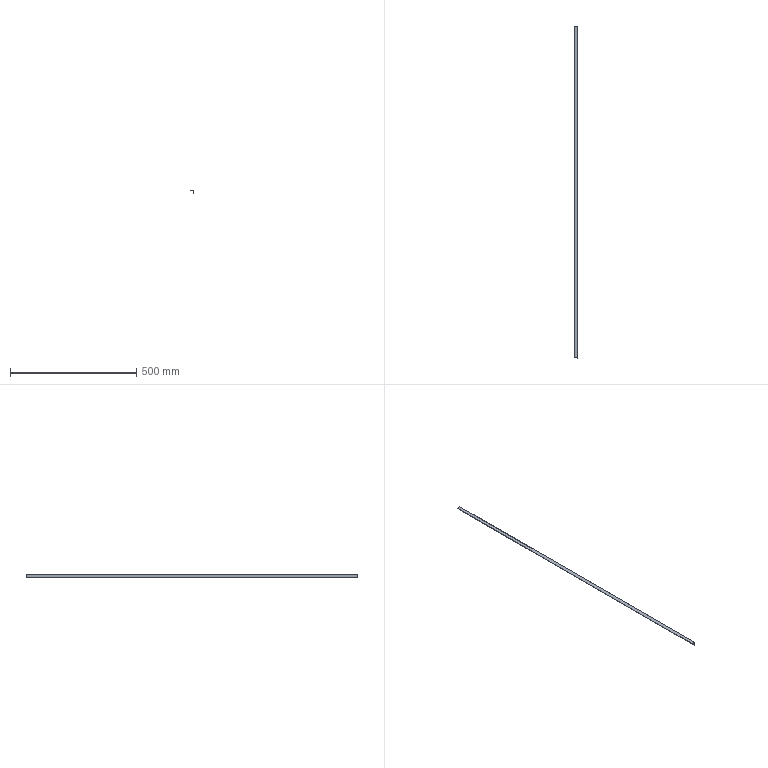Part | SolidWorks | features SplitBody 1 | 1 solid | 14 faces | box 15 x 1317 x 15 mm | volume 37839 mm3 | plane 12 | cylinder 2 | commonest cylinder face diameters 0.2 x1 2.2 x1
STEP:
#1=CARTESIAN_POINT('',(-434.9,1437.5,298.8));
#2=VERTEX_POINT('',#1);
#3=CARTESIAN_POINT('',(-434.9,1437.5,297.8));
#4=VERTEX_POINT('',#3);
#5=CARTESIAN_POINT('',(-434.9,1437.5,298.8));
#6=DIRECTION('',(0.,0.,-1.));
#7=VECTOR('',#6,1000.);
#8=LINE('',#5,#7);
#9=EDGE_CURVE('',#2,#4,#8,.T.);
#10=ORIENTED_EDGE('',*,*,#9,.F.);
#11=CARTESIAN_POINT('',(-433.8,1437.5,297.7));
#12=VERTEX_POINT('',#11);
#13=CARTESIAN_POINT('',(-434.9,1437.5,297.7));
#14=DIRECTION('',(0.,1.,0.));
#15=DIRECTION('',(0.,0.,1.));
#16=AXIS2_PLACEMENT_3D('',#13,#14,#15);
#17=CIRCLE('',#16,1.1);
#18=EDGE_CURVE('',#2,#12,#17,.T.);
#19=ORIENTED_EDGE('',*,*,#18,.T.);
#20=CARTESIAN_POINT('',(-434.8,1437.5,297.7));
#21=VERTEX_POINT('',#20);
#22=CARTESIAN_POINT('',(-434.8,1437.5,297.7));
#23=DIRECTION('',(1.,0.,0.));
#24=VECTOR('',#23,1000.);
#25=LINE('',#22,#24);
#26=EDGE_CURVE('',#21,#12,#25,.T.);
#27=ORIENTED_EDGE('',*,*,#26,.F.);
#28=CARTESIAN_POINT('',(-434.9,1437.5,297.7));
#29=DIRECTION('',(0.,1.,0.));
#30=DIRECTION('',(1.,0.,0.));
#31=AXIS2_PLACEMENT_3D('',#28,#29,#30);
#32=CIRCLE('',#31,0.1);
#33=EDGE_CURVE('',#4,#21,#32,.T.);
#34=ORIENTED_EDGE('',*,*,#33,.F.);
#35=EDGE_LOOP('',(#10,#19,#27,#34));
#36=FACE_OUTER_BOUND('',#35,.T.);
#37=CARTESIAN_POINT('',(-434.9,1437.5,298.8));
#38=DIRECTION('',(0.,1.,0.));
#39=DIRECTION('',(0.,0.,1.));
#40=AXIS2_PLACEMENT_3D('',#37,#38,#39);
#41=PLANE('',#40);
#42=ADVANCED_FACE('',(#36),#41,.T.);
#43=CARTESIAN_POINT('',(-448.8,1437.5,298.8));
#44=VERTEX_POINT('',#43);
#45=CARTESIAN_POINT('',(-433.8,1437.5,298.8));
#46=DIRECTION('',(1.,0.,0.));
#47=VECTOR('',#46,1000.);
#48=LINE('',#45,#47);
#49=EDGE_CURVE('',#44,#2,#48,.T.);
#50=ORIENTED_EDGE('',*,*,#49,.T.);
#51=ORIENTED_EDGE('',*,*,#9,.T.);
#52=CARTESIAN_POINT('',(-448.8,1437.5,297.8));
#53=VERTEX_POINT('',#52);
#54=CARTESIAN_POINT('',(-433.8,1437.5,297.8));
#55=DIRECTION('',(1.,0.,0.));
#56=VECTOR('',#55,1000.);
#57=LINE('',#54,#56);
#58=EDGE_CURVE('',#53,#4,#57,.T.);
#59=ORIENTED_EDGE('',*,*,#58,.F.);
#60=CARTESIAN_POINT('',(-448.8,1437.5,297.8));
#61=DIRECTION('',(0.,0.,1.));
#62=VECTOR('',#61,1000.);
#63=LINE('',#60,#62);
#64=EDGE_CURVE('',#53,#44,#63,.T.);
#65=ORIENTED_EDGE('',*,*,#64,.T.);
#66=EDGE_LOOP('',(#50,#51,#59,#65));
#67=FACE_OUTER_BOUND('',#66,.T.);
#68=CARTESIAN_POINT('',(-434.8,1437.5,297.7));
#69=DIRECTION('',(0.,1.,0.));
#70=DIRECTION('',(0.,0.,1.));
#71=AXIS2_PLACEMENT_3D('',#68,#69,#70);
#72=PLANE('',#71);
#73=ADVANCED_FACE('',(#67),#72,.T.);
#74=CARTESIAN_POINT('',(-434.8,121.,283.8));
#75=VERTEX_POINT('',#74);
#76=CARTESIAN_POINT('',(-434.8,121.,297.7));
#77=VERTEX_POINT('',#76);
#78=CARTESIAN_POINT('',(-434.8,121.,298.8));
#79=DIRECTION('',(0.,0.,1.));
#80=VECTOR('',#79,1000.);
#81=LINE('',#78,#80);
#82=EDGE_CURVE('',#75,#77,#81,.T.);
#83=ORIENTED_EDGE('',*,*,#82,.T.);
#84=CARTESIAN_POINT('',(-434.8,99.787,297.7));
#85=DIRECTION('',(0.,1.,0.));
#86=VECTOR('',#85,1000.);
#87=LINE('',#84,#86);
#88=EDGE_CURVE('',#77,#21,#87,.T.);
#89=ORIENTED_EDGE('',*,*,#88,.T.);
#90=CARTESIAN_POINT('',(-434.8,1437.5,283.8));
#91=VERTEX_POINT('',#90);
#92=CARTESIAN_POINT('',(-434.8,1437.5,298.8));
#93=DIRECTION('',(0.,0.,-1.));
#94=VECTOR('',#93,1000.);
#95=LINE('',#92,#94);
#96=EDGE_CURVE('',#21,#91,#95,.T.);
#97=ORIENTED_EDGE('',*,*,#96,.T.);
#98=CARTESIAN_POINT('',(-434.8,99.787,283.8));
#99=DIRECTION('',(0.,1.,0.));
#100=VECTOR('',#99,1000.);
#101=LINE('',#98,#100);
#102=EDGE_CURVE('',#75,#91,#101,.T.);
#103=ORIENTED_EDGE('',*,*,#102,.F.);
#104=EDGE_LOOP('',(#83,#89,#97,#103));
#105=FACE_OUTER_BOUND('',#104,.T.);
#106=CARTESIAN_POINT('',(-434.8,99.787,298.8));
#107=DIRECTION('',(1.,0.,0.));
#108=DIRECTION('',(0.,1.,0.));
#109=AXIS2_PLACEMENT_3D('',#106,#107,#108);
#110=PLANE('',#109);
#111=ADVANCED_FACE('',(#105),#110,.F.);
#112=CARTESIAN_POINT('',(-433.8,121.,283.8));
#113=VERTEX_POINT('',#112);
#114=CARTESIAN_POINT('',(-433.8,1437.5,283.8));
#115=VERTEX_POINT('',#114);
#116=CARTESIAN_POINT('',(-433.8,99.787,283.8));
#117=DIRECTION('',(0.,1.,0.));
#118=VECTOR('',#117,1000.);
#119=LINE('',#116,#118);
#120=EDGE_CURVE('',#113,#115,#119,.T.);
#121=ORIENTED_EDGE('',*,*,#120,.F.);
#122=CARTESIAN_POINT('',(-434.8,121.,283.8));
#123=DIRECTION('',(1.,0.,0.));
#124=VECTOR('',#123,1000.);
#125=LINE('',#122,#124);
#126=EDGE_CURVE('',#75,#113,#125,.T.);
#127=ORIENTED_EDGE('',*,*,#126,.F.);
#128=ORIENTED_EDGE('',*,*,#102,.T.);
#129=CARTESIAN_POINT('',(-433.8,1437.5,283.8));
#130=DIRECTION('',(-1.,0.,0.));
#131=VECTOR('',#130,1000.);
#132=LINE('',#129,#131);
#133=EDGE_CURVE('',#115,#91,#132,.T.);
#134=ORIENTED_EDGE('',*,*,#133,.F.);
#135=EDGE_LOOP('',(#121,#127,#128,#134));
#136=FACE_OUTER_BOUND('',#135,.T.);
#137=CARTESIAN_POINT('',(-433.8,99.787,283.8));
#138=DIRECTION('',(0.,0.,-1.));
#139=DIRECTION('',(-1.,0.,0.));
#140=AXIS2_PLACEMENT_3D('',#137,#138,#139);
#141=PLANE('',#140);
#142=ADVANCED_FACE('',(#136),#141,.T.);
#143=CARTESIAN_POINT('',(-433.8,121.,297.7));
#144=VERTEX_POINT('',#143);
#145=CARTESIAN_POINT('',(-433.8,99.787,297.7));
#146=DIRECTION('',(0.,1.,0.));
#147=VECTOR('',#146,1000.);
#148=LINE('',#145,#147);
#149=EDGE_CURVE('',#144,#12,#148,.T.);
#150=ORIENTED_EDGE('',*,*,#149,.F.);
#151=CARTESIAN_POINT('',(-433.8,121.,298.8));
#152=DIRECTION('',(0.,0.,1.));
#153=VECTOR('',#152,1000.);
#154=LINE('',#151,#153);
#155=EDGE_CURVE('',#113,#144,#154,.T.);
#156=ORIENTED_EDGE('',*,*,#155,.F.);
#157=ORIENTED_EDGE('',*,*,#120,.T.);
#158=CARTESIAN_POINT('',(-433.8,1437.5,298.8));
#159=DIRECTION('',(0.,0.,-1.));
#160=VECTOR('',#159,1000.);
#161=LINE('',#158,#160);
#162=EDGE_CURVE('',#12,#115,#161,.T.);
#163=ORIENTED_EDGE('',*,*,#162,.F.);
#164=EDGE_LOOP('',(#150,#156,#157,#163));
#165=FACE_OUTER_BOUND('',#164,.T.);
#166=CARTESIAN_POINT('',(-433.8,99.787,298.8));
#167=DIRECTION('',(1.,0.,0.));
#168=DIRECTION('',(0.,1.,0.));
#169=AXIS2_PLACEMENT_3D('',#166,#167,#168);
#170=PLANE('',#169);
#171=ADVANCED_FACE('',(#165),#170,.T.);
#172=CARTESIAN_POINT('',(-434.9,121.,298.8));
#173=VERTEX_POINT('',#172);
#174=CARTESIAN_POINT('',(-434.9,99.787,298.8));
#175=DIRECTION('',(0.,1.,0.));
#176=VECTOR('',#175,1000.);
#177=LINE('',#174,#176);
#178=EDGE_CURVE('',#173,#2,#177,.T.);
#179=ORIENTED_EDGE('',*,*,#178,.F.);
#180=CARTESIAN_POINT('',(-434.9,121.,297.7));
#181=DIRECTION('',(0.,-1.,0.));
#182=DIRECTION('',(1.,0.,0.));
#183=AXIS2_PLACEMENT_3D('',#180,#181,#182);
#184=CIRCLE('',#183,1.1);
#185=EDGE_CURVE('',#144,#173,#184,.T.);
#186=ORIENTED_EDGE('',*,*,#185,.F.);
#187=ORIENTED_EDGE('',*,*,#149,.T.);
#188=ORIENTED_EDGE('',*,*,#18,.F.);
#189=EDGE_LOOP('',(#179,#186,#187,#188));
#190=FACE_OUTER_BOUND('',#189,.T.);
#191=CARTESIAN_POINT('',(-434.9,99.787,297.7));
#192=DIRECTION('',(0.,1.,0.));
#193=DIRECTION('',(-1.,0.,0.));
#194=AXIS2_PLACEMENT_3D('',#191,#192,#193);
#195=CYLINDRICAL_SURFACE('',#194,1.1);
#196=ADVANCED_FACE('',(#190),#195,.T.);
#197=CARTESIAN_POINT('',(-448.8,121.,298.8));
#198=VERTEX_POINT('',#197);
#199=CARTESIAN_POINT('',(-448.8,99.787,298.8));
#200=DIRECTION('',(0.,1.,0.));
#201=VECTOR('',#200,1000.);
#202=LINE('',#199,#201);
#203=EDGE_CURVE('',#198,#44,#202,.T.);
#204=ORIENTED_EDGE('',*,*,#203,.F.);
#205=CARTESIAN_POINT('',(-433.8,121.,298.8));
#206=DIRECTION('',(-1.,0.,0.));
#207=VECTOR('',#206,1000.);
#208=LINE('',#205,#207);
#209=EDGE_CURVE('',#173,#198,#208,.T.);
#210=ORIENTED_EDGE('',*,*,#209,.F.);
#211=ORIENTED_EDGE('',*,*,#178,.T.);
#212=ORIENTED_EDGE('',*,*,#49,.F.);
#213=EDGE_LOOP('',(#204,#210,#211,#212));
#214=FACE_OUTER_BOUND('',#213,.T.);
#215=CARTESIAN_POINT('',(-433.8,99.787,298.8));
#216=DIRECTION('',(0.,0.,1.));
#217=DIRECTION('',(1.,0.,0.));
#218=AXIS2_PLACEMENT_3D('',#215,#216,#217);
#219=PLANE('',#218);
#220=ADVANCED_FACE('',(#214),#219,.T.);
#221=CARTESIAN_POINT('',(-448.8,121.,297.8));
#222=VERTEX_POINT('',#221);
#223=CARTESIAN_POINT('',(-448.8,99.787,297.8));
#224=DIRECTION('',(0.,1.,0.));
#225=VECTOR('',#224,1000.);
#226=LINE('',#223,#225);
#227=EDGE_CURVE('',#222,#53,#226,.T.);
#228=ORIENTED_EDGE('',*,*,#227,.F.);
#229=CARTESIAN_POINT('',(-448.8,121.,297.8));
#230=DIRECTION('',(0.,0.,1.));
#231=VECTOR('',#230,1000.);
#232=LINE('',#229,#231);
#233=EDGE_CURVE('',#222,#198,#232,.T.);
#234=ORIENTED_EDGE('',*,*,#233,.T.);
#235=ORIENTED_EDGE('',*,*,#203,.T.);
#236=ORIENTED_EDGE('',*,*,#64,.F.);
#237=EDGE_LOOP('',(#228,#234,#235,#236));
#238=FACE_OUTER_BOUND('',#237,.T.);
#239=CARTESIAN_POINT('',(-448.8,99.787,297.8));
#240=DIRECTION('',(-1.,0.,0.));
#241=DIRECTION('',(0.,-1.,0.));
#242=AXIS2_PLACEMENT_3D('',#239,#240,#241);
#243=PLANE('',#242);
#244=ADVANCED_FACE('',(#238),#243,.T.);
#245=CARTESIAN_POINT('',(-434.9,121.,297.8));
#246=VERTEX_POINT('',#245);
#247=CARTESIAN_POINT('',(-433.8,121.,297.8));
#248=DIRECTION('',(-1.,0.,0.));
#249=VECTOR('',#248,1000.);
#250=LINE('',#247,#249);
#251=EDGE_CURVE('',#246,#222,#250,.T.);
#252=ORIENTED_EDGE('',*,*,#251,.T.);
#253=ORIENTED_EDGE('',*,*,#227,.T.);
#254=ORIENTED_EDGE('',*,*,#58,.T.);
#255=CARTESIAN_POINT('',(-434.9,99.787,297.8));
#256=DIRECTION('',(0.,1.,0.));
#257=VECTOR('',#256,1000.);
#258=LINE('',#255,#257);
#259=EDGE_CURVE('',#246,#4,#258,.T.);
#260=ORIENTED_EDGE('',*,*,#259,.F.);
#261=EDGE_LOOP('',(#252,#253,#254,#260));
#262=FACE_OUTER_BOUND('',#261,.T.);
#263=CARTESIAN_POINT('',(-433.8,99.787,297.8));
#264=DIRECTION('',(0.,0.,1.));
#265=DIRECTION('',(1.,0.,0.));
#266=AXIS2_PLACEMENT_3D('',#263,#264,#265);
#267=PLANE('',#266);
#268=ADVANCED_FACE('',(#262),#267,.F.);
#269=CARTESIAN_POINT('',(-434.9,121.,297.7));
#270=DIRECTION('',(0.,-1.,0.));
#271=DIRECTION('',(-1.,0.,0.));
#272=AXIS2_PLACEMENT_3D('',#269,#270,#271);
#273=CIRCLE('',#272,0.1);
#274=EDGE_CURVE('',#77,#246,#273,.T.);
#275=ORIENTED_EDGE('',*,*,#274,.T.);
#276=ORIENTED_EDGE('',*,*,#259,.T.);
#277=ORIENTED_EDGE('',*,*,#33,.T.);
#278=ORIENTED_EDGE('',*,*,#88,.F.);
#279=EDGE_LOOP('',(#275,#276,#277,#278));
#280=FACE_OUTER_BOUND('',#279,.T.);
#281=CARTESIAN_POINT('',(-434.9,99.787,297.7));
#282=DIRECTION('',(0.,1.,0.));
#283=DIRECTION('',(-1.,0.,0.));
#284=AXIS2_PLACEMENT_3D('',#281,#282,#283);
#285=CYLINDRICAL_SURFACE('',#284,0.1);
#286=ADVANCED_FACE('',(#280),#285,.F.);
#287=ORIENTED_EDGE('',*,*,#96,.F.);
#288=ORIENTED_EDGE('',*,*,#26,.T.);
#289=ORIENTED_EDGE('',*,*,#162,.T.);
#290=ORIENTED_EDGE('',*,*,#133,.T.);
#291=EDGE_LOOP('',(#287,#288,#289,#290));
#292=FACE_OUTER_BOUND('',#291,.T.);
#293=CARTESIAN_POINT('',(-434.9,1437.5,297.7));
#294=DIRECTION('',(0.,1.,0.));
#295=DIRECTION('',(-1.,0.,0.));
#296=AXIS2_PLACEMENT_3D('',#293,#294,#295);
#297=PLANE('',#296);
#298=ADVANCED_FACE('',(#292),#297,.T.);
#299=CARTESIAN_POINT('',(-434.8,121.,297.7));
#300=DIRECTION('',(1.,0.,0.));
#301=VECTOR('',#300,1000.);
#302=LINE('',#299,#301);
#303=EDGE_CURVE('',#77,#144,#302,.T.);
#304=ORIENTED_EDGE('',*,*,#303,.F.);
#305=ORIENTED_EDGE('',*,*,#82,.F.);
#306=ORIENTED_EDGE('',*,*,#126,.T.);
#307=ORIENTED_EDGE('',*,*,#155,.T.);
#308=EDGE_LOOP('',(#304,#305,#306,#307));
#309=FACE_OUTER_BOUND('',#308,.T.);
#310=CARTESIAN_POINT('',(-434.8,121.,298.8));
#311=DIRECTION('',(0.,1.,0.));
#312=DIRECTION('',(0.,0.,1.));
#313=AXIS2_PLACEMENT_3D('',#310,#311,#312);
#314=PLANE('',#313);
#315=ADVANCED_FACE('',(#309),#314,.F.);
#316=ORIENTED_EDGE('',*,*,#233,.F.);
#317=ORIENTED_EDGE('',*,*,#251,.F.);
#318=CARTESIAN_POINT('',(-434.9,121.,297.8));
#319=DIRECTION('',(0.,0.,1.));
#320=VECTOR('',#319,1000.);
#321=LINE('',#318,#320);
#322=EDGE_CURVE('',#246,#173,#321,.T.);
#323=ORIENTED_EDGE('',*,*,#322,.T.);
#324=ORIENTED_EDGE('',*,*,#209,.T.);
#325=EDGE_LOOP('',(#316,#317,#323,#324));
#326=FACE_OUTER_BOUND('',#325,.T.);
#327=CARTESIAN_POINT('',(-433.8,121.,297.8));
#328=DIRECTION('',(0.,1.,0.));
#329=DIRECTION('',(-1.,0.,0.));
#330=AXIS2_PLACEMENT_3D('',#327,#328,#329);
#331=PLANE('',#330);
#332=ADVANCED_FACE('',(#326),#331,.F.);
#333=ORIENTED_EDGE('',*,*,#185,.T.);
#334=ORIENTED_EDGE('',*,*,#322,.F.);
#335=ORIENTED_EDGE('',*,*,#274,.F.);
#336=ORIENTED_EDGE('',*,*,#303,.T.);
#337=EDGE_LOOP('',(#333,#334,#335,#336));
#338=FACE_OUTER_BOUND('',#337,.T.);
#339=CARTESIAN_POINT('',(-434.9,121.,297.7));
#340=DIRECTION('',(0.,-1.,0.));
#341=DIRECTION('',(1.,0.,0.));
#342=AXIS2_PLACEMENT_3D('',#339,#340,#341);
#343=PLANE('',#342);
#344=ADVANCED_FACE('',(#338),#343,.T.);
#345=CLOSED_SHELL('',(#42,#73,#111,#142,#171,#196,#220,#244,#268,#286,#298,#315,#332,#344));
#346=MANIFOLD_SOLID_BREP('',#345);
#347=CARTESIAN_POINT('',(0.,0.,0.));
#348=DIRECTION('',(0.,0.,1.));
#349=DIRECTION('',(1.,0.,0.));
#350=AXIS2_PLACEMENT_3D('',#347,#348,#349);
#351=(LENGTH_UNIT()NAMED_UNIT(*)SI_UNIT(.MILLI.,.METRE.));
#352=UNCERTAINTY_MEASURE_WITH_UNIT(LENGTH_MEASURE(0.00001),#351,'','');
#353=(NAMED_UNIT(*)PLANE_ANGLE_UNIT()SI_UNIT($,.RADIAN.));
#354=(NAMED_UNIT(*)SI_UNIT($,.STERADIAN.)SOLID_ANGLE_UNIT());
#355=(GEOMETRIC_REPRESENTATION_CONTEXT(3)GLOBAL_UNCERTAINTY_ASSIGNED_CONTEXT((#352))GLOBAL_UNIT_ASSIGNED_CONTEXT((#351,#353,#354))REPRESENTATION_CONTEXT('',''));
#356=ADVANCED_BREP_SHAPE_REPRESENTATION('',(#346,#350),#355);